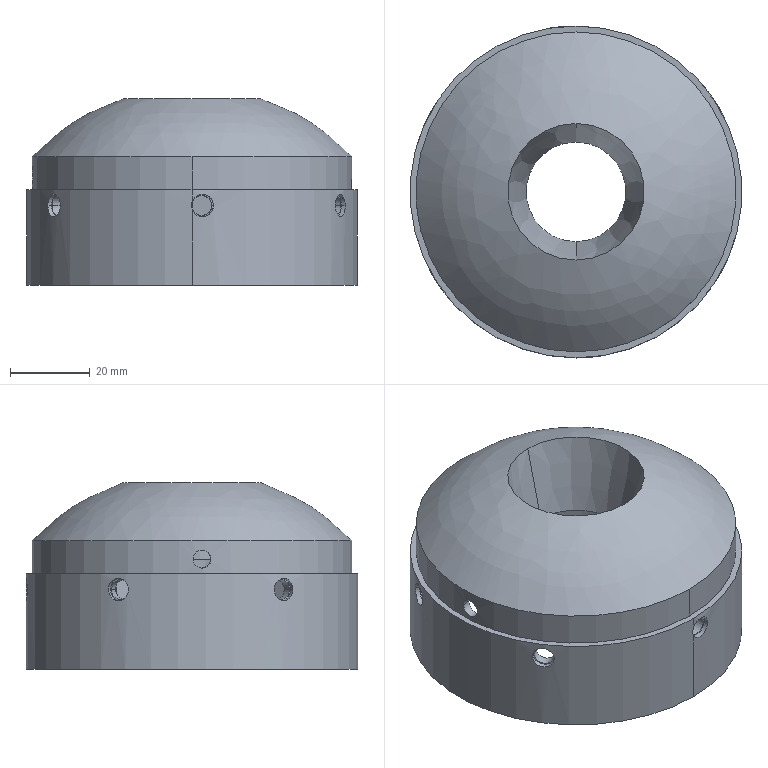Part | SolidWorks | features BaseBody 1 | 1 solid | 49 faces | box 83 x 83 x 46.77 mm | volume 58968 mm3 | cylinder 34 | plane 10 | cone 4 | spline 1 | commonest cylinder face diameters 5 x12 5.6 x12 4.5 x2 33 x2 76 x2 80 x2